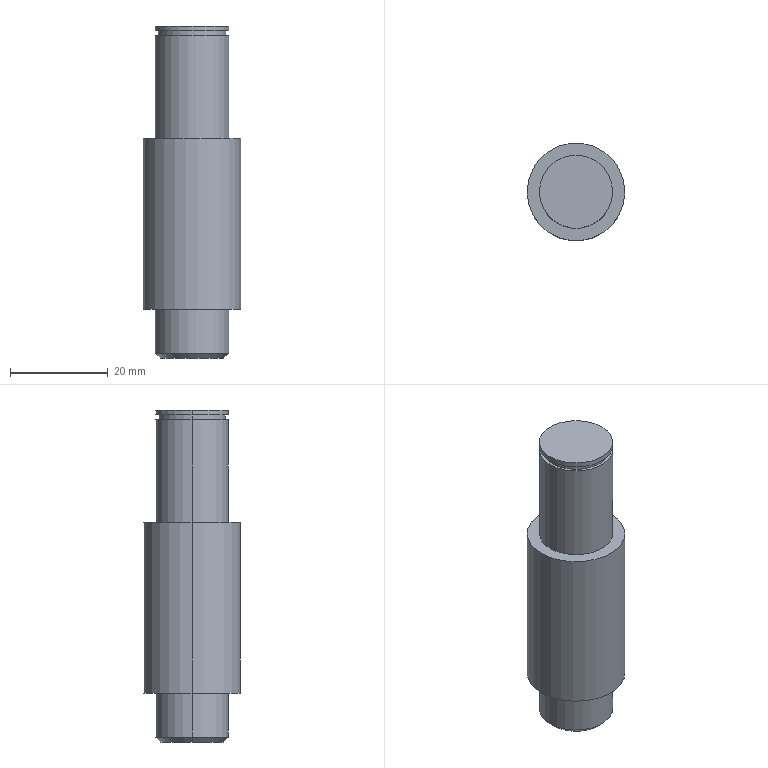Part | STEP file | Tensioning pulley fixing shaft SGN-2-20 | 1 solid | 18 faces | box 20 x 20 x 68 mm | volume 16777 mm3 | cylinder 10 | plane 6 | cone 2 | commonest cylinder face diameters 15 x6 13.8 x2 20 x2
STEP:
#1=CARTESIAN_POINT('',(0.,0.,0.));
#2=DIRECTION('',(0.,0.,1.));
#3=DIRECTION('',(1.,0.,0.));
#4=AXIS2_PLACEMENT_3D('',#1,#2,#3);
#5=CARTESIAN_POINT('',(-6.5,0.,0.));
#6=VERTEX_POINT('',#5);
#7=CARTESIAN_POINT('',(6.5,0.,0.));
#8=VERTEX_POINT('',#7);
#9=CARTESIAN_POINT('',(0.,0.,0.));
#10=DIRECTION('',(0.,0.,-1.));
#11=DIRECTION('',(1.,0.,0.));
#12=AXIS2_PLACEMENT_3D('',#9,#10,#11);
#13=CIRCLE('',#12,6.5);
#14=CARTESIAN_POINT('',(0.,0.,1.));
#15=DIRECTION('',(0.,0.,1.));
#16=DIRECTION('',(1.,0.,0.));
#17=AXIS2_PLACEMENT_3D('',#14,#15,#16);
#18=CONICAL_SURFACE('',#17,7.5,0.7854);
#19=CARTESIAN_POINT('',(6.283,-1.));
#20=DIRECTION('',(-1.,0.));
#21=VECTOR('',#20,1.);
#22=LINE('',#19,#21);
#23=(GEOMETRIC_REPRESENTATION_CONTEXT(2)PARAMETRIC_REPRESENTATION_CONTEXT()REPRESENTATION_CONTEXT('',''));
#24=DEFINITIONAL_REPRESENTATION('',(#22),#23);
#25=PCURVE('',#18,#24);
#26=CARTESIAN_POINT('',(0.,0.,0.));
#27=DIRECTION('',(0.,0.,1.));
#28=DIRECTION('',(1.,0.,0.));
#29=AXIS2_PLACEMENT_3D('',#26,#27,#28);
#30=PLANE('',#29);
#31=CARTESIAN_POINT('',(6.5,0.));
#32=CARTESIAN_POINT('',(6.5,-11.258));
#33=CARTESIAN_POINT('',(-3.25,-5.629));
#34=CARTESIAN_POINT('',(-13.,0.));
#35=CARTESIAN_POINT('',(-3.25,5.629));
#36=CARTESIAN_POINT('',(6.5,11.258));
#37=CARTESIAN_POINT('',(6.5,0.));
#38=(BOUNDED_CURVE()B_SPLINE_CURVE(2,(#31,#32,#33,#34,#35,#36,#37),.UNSPECIFIED.,.T.,.F.)B_SPLINE_CURVE_WITH_KNOTS((1,2,2,2,2,1),(-2.094,0.,2.094,4.189,6.283,8.378),.UNSPECIFIED.)CURVE()GEOMETRIC_REPRESENTATION_ITEM()RATIONAL_B_SPLINE_CURVE((1.,0.5,1.,0.5,1.,0.5,1.))REPRESENTATION_ITEM(''));
#39=(GEOMETRIC_REPRESENTATION_CONTEXT(2)PARAMETRIC_REPRESENTATION_CONTEXT()REPRESENTATION_CONTEXT('',''));
#40=DEFINITIONAL_REPRESENTATION('',(#38),#39);
#41=PCURVE('',#30,#40);
#42=SURFACE_CURVE('',#13,(#25,#41),.PCURVE_S1.);
#43=EDGE_CURVE('',#6,#8,#42,.T.);
#44=ORIENTED_EDGE('',*,*,#43,.F.);
#45=CARTESIAN_POINT('',(-7.5,0.,1.));
#46=VERTEX_POINT('',#45);
#47=CARTESIAN_POINT('',(-7.5,0.,1.));
#48=DIRECTION('',(-0.7071,0.,0.7071));
#49=VECTOR('',#48,1.);
#50=LINE('',#47,#49);
#51=CARTESIAN_POINT('',(3.142,0.));
#52=DIRECTION('',(0.,1.));
#53=VECTOR('',#52,1.);
#54=LINE('',#51,#53);
#55=(GEOMETRIC_REPRESENTATION_CONTEXT(2)PARAMETRIC_REPRESENTATION_CONTEXT()REPRESENTATION_CONTEXT('',''));
#56=DEFINITIONAL_REPRESENTATION('',(#54),#55);
#57=PCURVE('',#18,#56);
#58=CARTESIAN_POINT('',(0.,0.,1.));
#59=DIRECTION('',(0.,0.,1.));
#60=DIRECTION('',(1.,0.,0.));
#61=AXIS2_PLACEMENT_3D('',#58,#59,#60);
#62=CONICAL_SURFACE('',#61,7.5,0.7854);
#63=CARTESIAN_POINT('',(3.142,0.));
#64=DIRECTION('',(0.,1.));
#65=VECTOR('',#64,1.);
#66=LINE('',#63,#65);
#67=(GEOMETRIC_REPRESENTATION_CONTEXT(2)PARAMETRIC_REPRESENTATION_CONTEXT()REPRESENTATION_CONTEXT('',''));
#68=DEFINITIONAL_REPRESENTATION('',(#66),#67);
#69=PCURVE('',#62,#68);
#70=SURFACE_CURVE('',#50,(#57,#69),.PCURVE_S1.);
#71=EDGE_CURVE('',#6,#46,#70,.T.);
#72=ORIENTED_EDGE('',*,*,#71,.T.);
#73=CARTESIAN_POINT('',(7.5,0.,1.));
#74=VERTEX_POINT('',#73);
#75=CARTESIAN_POINT('',(0.,0.,1.));
#76=DIRECTION('',(0.,0.,1.));
#77=DIRECTION('',(1.,0.,0.));
#78=AXIS2_PLACEMENT_3D('',#75,#76,#77);
#79=CIRCLE('',#78,7.5);
#80=CARTESIAN_POINT('',(0.,0.));
#81=DIRECTION('',(1.,0.));
#82=VECTOR('',#81,1.);
#83=LINE('',#80,#82);
#84=(GEOMETRIC_REPRESENTATION_CONTEXT(2)PARAMETRIC_REPRESENTATION_CONTEXT()REPRESENTATION_CONTEXT('',''));
#85=DEFINITIONAL_REPRESENTATION('',(#83),#84);
#86=PCURVE('',#18,#85);
#87=CARTESIAN_POINT('',(0.,0.,10.));
#88=DIRECTION('',(0.,0.,-1.));
#89=DIRECTION('',(-1.,0.,0.));
#90=AXIS2_PLACEMENT_3D('',#87,#88,#89);
#91=CYLINDRICAL_SURFACE('',#90,7.5);
#92=CARTESIAN_POINT('',(3.142,9.));
#93=DIRECTION('',(-1.,0.));
#94=VECTOR('',#93,1.);
#95=LINE('',#92,#94);
#96=(GEOMETRIC_REPRESENTATION_CONTEXT(2)PARAMETRIC_REPRESENTATION_CONTEXT()REPRESENTATION_CONTEXT('',''));
#97=DEFINITIONAL_REPRESENTATION('',(#95),#96);
#98=PCURVE('',#91,#97);
#99=SURFACE_CURVE('',#79,(#86,#98),.PCURVE_S1.);
#100=EDGE_CURVE('',#74,#46,#99,.T.);
#101=ORIENTED_EDGE('',*,*,#100,.F.);
#102=CARTESIAN_POINT('',(7.5,0.,1.));
#103=DIRECTION('',(0.7071,0.,0.7071));
#104=VECTOR('',#103,1.);
#105=LINE('',#102,#104);
#106=CARTESIAN_POINT('',(0.,0.));
#107=DIRECTION('',(0.,1.));
#108=VECTOR('',#107,1.);
#109=LINE('',#106,#108);
#110=(GEOMETRIC_REPRESENTATION_CONTEXT(2)PARAMETRIC_REPRESENTATION_CONTEXT()REPRESENTATION_CONTEXT('',''));
#111=DEFINITIONAL_REPRESENTATION('',(#109),#110);
#112=PCURVE('',#18,#111);
#113=CARTESIAN_POINT('',(6.283,0.));
#114=DIRECTION('',(0.,1.));
#115=VECTOR('',#114,1.);
#116=LINE('',#113,#115);
#117=(GEOMETRIC_REPRESENTATION_CONTEXT(2)PARAMETRIC_REPRESENTATION_CONTEXT()REPRESENTATION_CONTEXT('',''));
#118=DEFINITIONAL_REPRESENTATION('',(#116),#117);
#119=PCURVE('',#62,#118);
#120=SURFACE_CURVE('',#105,(#112,#119),.PCURVE_S1.);
#121=EDGE_CURVE('',#8,#74,#120,.T.);
#122=ORIENTED_EDGE('',*,*,#121,.F.);
#123=EDGE_LOOP('',(#44,#72,#101,#122));
#124=FACE_BOUND('',#123,.T.);
#125=ADVANCED_FACE('',(#124),#18,.T.);
#126=CARTESIAN_POINT('',(7.5,0.,68.));
#127=VERTEX_POINT('',#126);
#128=CARTESIAN_POINT('',(-7.5,0.,68.));
#129=VERTEX_POINT('',#128);
#130=CARTESIAN_POINT('',(0.,0.,68.));
#131=DIRECTION('',(0.,0.,1.));
#132=DIRECTION('',(1.,0.,0.));
#133=AXIS2_PLACEMENT_3D('',#130,#131,#132);
#134=CIRCLE('',#133,7.5);
#135=CARTESIAN_POINT('',(0.,0.,68.));
#136=DIRECTION('',(0.,0.,-1.));
#137=DIRECTION('',(-1.,0.,0.));
#138=AXIS2_PLACEMENT_3D('',#135,#136,#137);
#139=CYLINDRICAL_SURFACE('',#138,7.5);
#140=CARTESIAN_POINT('',(3.142,0.));
#141=DIRECTION('',(-1.,0.));
#142=VECTOR('',#141,1.);
#143=LINE('',#140,#142);
#144=(GEOMETRIC_REPRESENTATION_CONTEXT(2)PARAMETRIC_REPRESENTATION_CONTEXT()REPRESENTATION_CONTEXT('',''));
#145=DEFINITIONAL_REPRESENTATION('',(#143),#144);
#146=PCURVE('',#139,#145);
#147=CARTESIAN_POINT('',(0.,0.,68.));
#148=DIRECTION('',(0.,0.,1.));
#149=DIRECTION('',(1.,0.,0.));
#150=AXIS2_PLACEMENT_3D('',#147,#148,#149);
#151=PLANE('',#150);
#152=CARTESIAN_POINT('',(0.,0.));
#153=DIRECTION('',(1.,0.));
#154=AXIS2_PLACEMENT_2D('',#152,#153);
#155=CIRCLE('',#154,7.5);
#156=(GEOMETRIC_REPRESENTATION_CONTEXT(2)PARAMETRIC_REPRESENTATION_CONTEXT()REPRESENTATION_CONTEXT('',''));
#157=DEFINITIONAL_REPRESENTATION('',(#155),#156);
#158=PCURVE('',#151,#157);
#159=SURFACE_CURVE('',#134,(#146,#158),.PCURVE_S1.);
#160=EDGE_CURVE('',#127,#129,#159,.T.);
#161=ORIENTED_EDGE('',*,*,#160,.F.);
#162=CARTESIAN_POINT('',(7.5,0.,67.));
#163=VERTEX_POINT('',#162);
#164=CARTESIAN_POINT('',(7.5,0.,68.));
#165=DIRECTION('',(0.,0.,-1.));
#166=VECTOR('',#165,1.);
#167=LINE('',#164,#166);
#168=CARTESIAN_POINT('',(3.142,0.));
#169=DIRECTION('',(0.,1.));
#170=VECTOR('',#169,1.);
#171=LINE('',#168,#170);
#172=(GEOMETRIC_REPRESENTATION_CONTEXT(2)PARAMETRIC_REPRESENTATION_CONTEXT()REPRESENTATION_CONTEXT('',''));
#173=DEFINITIONAL_REPRESENTATION('',(#171),#172);
#174=PCURVE('',#139,#173);
#175=CARTESIAN_POINT('',(0.,0.,68.));
#176=DIRECTION('',(0.,0.,-1.));
#177=DIRECTION('',(-1.,0.,0.));
#178=AXIS2_PLACEMENT_3D('',#175,#176,#177);
#179=CYLINDRICAL_SURFACE('',#178,7.5);
#180=CARTESIAN_POINT('',(3.142,0.));
#181=DIRECTION('',(0.,1.));
#182=VECTOR('',#181,1.);
#183=LINE('',#180,#182);
#184=(GEOMETRIC_REPRESENTATION_CONTEXT(2)PARAMETRIC_REPRESENTATION_CONTEXT()REPRESENTATION_CONTEXT('',''));
#185=DEFINITIONAL_REPRESENTATION('',(#183),#184);
#186=PCURVE('',#179,#185);
#187=SURFACE_CURVE('',#167,(#174,#186),.PCURVE_S1.);
#188=EDGE_CURVE('',#127,#163,#187,.T.);
#189=ORIENTED_EDGE('',*,*,#188,.T.);
#190=CARTESIAN_POINT('',(-7.5,0.,67.));
#191=VERTEX_POINT('',#190);
#192=CARTESIAN_POINT('',(0.,0.,67.));
#193=DIRECTION('',(0.,0.,1.));
#194=DIRECTION('',(1.,0.,0.));
#195=AXIS2_PLACEMENT_3D('',#192,#193,#194);
#196=CIRCLE('',#195,7.5);
#197=CARTESIAN_POINT('',(3.142,1.));
#198=DIRECTION('',(-1.,0.));
#199=VECTOR('',#198,1.);
#200=LINE('',#197,#199);
#201=(GEOMETRIC_REPRESENTATION_CONTEXT(2)PARAMETRIC_REPRESENTATION_CONTEXT()REPRESENTATION_CONTEXT('',''));
#202=DEFINITIONAL_REPRESENTATION('',(#200),#201);
#203=PCURVE('',#139,#202);
#204=CARTESIAN_POINT('',(0.,0.,67.));
#205=DIRECTION('',(0.,0.,1.));
#206=DIRECTION('',(1.,0.,0.));
#207=AXIS2_PLACEMENT_3D('',#204,#205,#206);
#208=PLANE('',#207);
#209=CARTESIAN_POINT('',(0.,0.));
#210=DIRECTION('',(1.,0.));
#211=AXIS2_PLACEMENT_2D('',#209,#210);
#212=CIRCLE('',#211,7.5);
#213=(GEOMETRIC_REPRESENTATION_CONTEXT(2)PARAMETRIC_REPRESENTATION_CONTEXT()REPRESENTATION_CONTEXT('',''));
#214=DEFINITIONAL_REPRESENTATION('',(#212),#213);
#215=PCURVE('',#208,#214);
#216=SURFACE_CURVE('',#196,(#203,#215),.PCURVE_S1.);
#217=EDGE_CURVE('',#163,#191,#216,.T.);
#218=ORIENTED_EDGE('',*,*,#217,.T.);
#219=CARTESIAN_POINT('',(-7.5,0.,68.));
#220=DIRECTION('',(0.,0.,-1.));
#221=VECTOR('',#220,1.);
#222=LINE('',#219,#221);
#223=CARTESIAN_POINT('',(0.,0.));
#224=DIRECTION('',(0.,1.));
#225=VECTOR('',#224,1.);
#226=LINE('',#223,#225);
#227=(GEOMETRIC_REPRESENTATION_CONTEXT(2)PARAMETRIC_REPRESENTATION_CONTEXT()REPRESENTATION_CONTEXT('',''));
#228=DEFINITIONAL_REPRESENTATION('',(#226),#227);
#229=PCURVE('',#139,#228);
#230=CARTESIAN_POINT('',(6.283,0.));
#231=DIRECTION('',(0.,1.));
#232=VECTOR('',#231,1.);
#233=LINE('',#230,#232);
#234=(GEOMETRIC_REPRESENTATION_CONTEXT(2)PARAMETRIC_REPRESENTATION_CONTEXT()REPRESENTATION_CONTEXT('',''));
#235=DEFINITIONAL_REPRESENTATION('',(#233),#234);
#236=PCURVE('',#179,#235);
#237=SURFACE_CURVE('',#222,(#229,#236),.PCURVE_S1.);
#238=EDGE_CURVE('',#129,#191,#237,.T.);
#239=ORIENTED_EDGE('',*,*,#238,.F.);
#240=EDGE_LOOP('',(#161,#189,#218,#239));
#241=FACE_BOUND('',#240,.T.);
#242=ADVANCED_FACE('',(#241),#139,.T.);
#243=CARTESIAN_POINT('',(6.9,0.,66.));
#244=VERTEX_POINT('',#243);
#245=CARTESIAN_POINT('',(-6.9,0.,66.));
#246=VERTEX_POINT('',#245);
#247=CARTESIAN_POINT('',(0.,0.,66.));
#248=DIRECTION('',(0.,0.,1.));
#249=DIRECTION('',(1.,0.,0.));
#250=AXIS2_PLACEMENT_3D('',#247,#248,#249);
#251=CIRCLE('',#250,6.9);
#252=CARTESIAN_POINT('',(0.,0.,66.));
#253=DIRECTION('',(0.,0.,1.));
#254=DIRECTION('',(1.,0.,0.));
#255=AXIS2_PLACEMENT_3D('',#252,#253,#254);
#256=CYLINDRICAL_SURFACE('',#255,6.9);
#257=CARTESIAN_POINT('',(0.,0.));
#258=DIRECTION('',(1.,0.));
#259=VECTOR('',#258,1.);
#260=LINE('',#257,#259);
#261=(GEOMETRIC_REPRESENTATION_CONTEXT(2)PARAMETRIC_REPRESENTATION_CONTEXT()REPRESENTATION_CONTEXT('',''));
#262=DEFINITIONAL_REPRESENTATION('',(#260),#261);
#263=PCURVE('',#256,#262);
#264=CARTESIAN_POINT('',(0.,0.,66.));
#265=DIRECTION('',(0.,0.,1.));
#266=DIRECTION('',(1.,0.,0.));
#267=AXIS2_PLACEMENT_3D('',#264,#265,#266);
#268=PLANE('',#267);
#269=CARTESIAN_POINT('',(0.,0.));
#270=DIRECTION('',(1.,0.));
#271=AXIS2_PLACEMENT_2D('',#269,#270);
#272=CIRCLE('',#271,6.9);
#273=(GEOMETRIC_REPRESENTATION_CONTEXT(2)PARAMETRIC_REPRESENTATION_CONTEXT()REPRESENTATION_CONTEXT('',''));
#274=DEFINITIONAL_REPRESENTATION('',(#272),#273);
#275=PCURVE('',#268,#274);
#276=SURFACE_CURVE('',#251,(#263,#275),.PCURVE_S1.);
#277=EDGE_CURVE('',#244,#246,#276,.T.);
#278=ORIENTED_EDGE('',*,*,#277,.T.);
#279=CARTESIAN_POINT('',(-6.9,0.,67.));
#280=VERTEX_POINT('',#279);
#281=CARTESIAN_POINT('',(-6.9,0.,66.));
#282=DIRECTION('',(0.,0.,1.));
#283=VECTOR('',#282,1.);
#284=LINE('',#281,#283);
#285=CARTESIAN_POINT('',(3.142,0.));
#286=DIRECTION('',(0.,1.));
#287=VECTOR('',#286,1.);
#288=LINE('',#285,#287);
#289=(GEOMETRIC_REPRESENTATION_CONTEXT(2)PARAMETRIC_REPRESENTATION_CONTEXT()REPRESENTATION_CONTEXT('',''));
#290=DEFINITIONAL_REPRESENTATION('',(#288),#289);
#291=PCURVE('',#256,#290);
#292=CARTESIAN_POINT('',(0.,0.,66.));
#293=DIRECTION('',(0.,0.,1.));
#294=DIRECTION('',(1.,0.,0.));
#295=AXIS2_PLACEMENT_3D('',#292,#293,#294);
#296=CYLINDRICAL_SURFACE('',#295,6.9);
#297=CARTESIAN_POINT('',(3.142,0.));
#298=DIRECTION('',(0.,1.));
#299=VECTOR('',#298,1.);
#300=LINE('',#297,#299);
#301=(GEOMETRIC_REPRESENTATION_CONTEXT(2)PARAMETRIC_REPRESENTATION_CONTEXT()REPRESENTATION_CONTEXT('',''));
#302=DEFINITIONAL_REPRESENTATION('',(#300),#301);
#303=PCURVE('',#296,#302);
#304=SURFACE_CURVE('',#284,(#291,#303),.PCURVE_S1.);
#305=EDGE_CURVE('',#246,#280,#304,.T.);
#306=ORIENTED_EDGE('',*,*,#305,.T.);
#307=CARTESIAN_POINT('',(6.9,0.,67.));
#308=VERTEX_POINT('',#307);
#309=CARTESIAN_POINT('',(0.,0.,67.));
#310=DIRECTION('',(0.,0.,1.));
#311=DIRECTION('',(1.,0.,0.));
#312=AXIS2_PLACEMENT_3D('',#309,#310,#311);
#313=CIRCLE('',#312,6.9);
#314=CARTESIAN_POINT('',(0.,1.));
#315=DIRECTION('',(1.,0.));
#316=VECTOR('',#315,1.);
#317=LINE('',#314,#316);
#318=(GEOMETRIC_REPRESENTATION_CONTEXT(2)PARAMETRIC_REPRESENTATION_CONTEXT()REPRESENTATION_CONTEXT('',''));
#319=DEFINITIONAL_REPRESENTATION('',(#317),#318);
#320=PCURVE('',#256,#319);
#321=CARTESIAN_POINT('',(0.,0.));
#322=DIRECTION('',(1.,0.));
#323=AXIS2_PLACEMENT_2D('',#321,#322);
#324=CIRCLE('',#323,6.9);
#325=(GEOMETRIC_REPRESENTATION_CONTEXT(2)PARAMETRIC_REPRESENTATION_CONTEXT()REPRESENTATION_CONTEXT('',''));
#326=DEFINITIONAL_REPRESENTATION('',(#324),#325);
#327=PCURVE('',#208,#326);
#328=SURFACE_CURVE('',#313,(#320,#327),.PCURVE_S1.);
#329=EDGE_CURVE('',#308,#280,#328,.T.);
#330=ORIENTED_EDGE('',*,*,#329,.F.);
#331=CARTESIAN_POINT('',(6.9,0.,66.));
#332=DIRECTION('',(0.,0.,1.));
#333=VECTOR('',#332,1.);
#334=LINE('',#331,#333);
#335=CARTESIAN_POINT('',(0.,0.));
#336=DIRECTION('',(0.,1.));
#337=VECTOR('',#336,1.);
#338=LINE('',#335,#337);
#339=(GEOMETRIC_REPRESENTATION_CONTEXT(2)PARAMETRIC_REPRESENTATION_CONTEXT()REPRESENTATION_CONTEXT('',''));
#340=DEFINITIONAL_REPRESENTATION('',(#338),#339);
#341=PCURVE('',#256,#340);
#342=CARTESIAN_POINT('',(6.283,0.));
#343=DIRECTION('',(0.,1.));
#344=VECTOR('',#343,1.);
#345=LINE('',#342,#344);
#346=(GEOMETRIC_REPRESENTATION_CONTEXT(2)PARAMETRIC_REPRESENTATION_CONTEXT()REPRESENTATION_CONTEXT('',''));
#347=DEFINITIONAL_REPRESENTATION('',(#345),#346);
#348=PCURVE('',#296,#347);
#349=SURFACE_CURVE('',#334,(#341,#348),.PCURVE_S1.);
#350=EDGE_CURVE('',#244,#308,#349,.T.);
#351=ORIENTED_EDGE('',*,*,#350,.F.);
#352=EDGE_LOOP('',(#278,#306,#330,#351));
#353=FACE_BOUND('',#352,.T.);
#354=ADVANCED_FACE('',(#353),#256,.T.);
#355=CARTESIAN_POINT('',(10.,0.,45.));
#356=VERTEX_POINT('',#355);
#357=CARTESIAN_POINT('',(-10.,0.,45.));
#358=VERTEX_POINT('',#357);
#359=CARTESIAN_POINT('',(0.,0.,45.));
#360=DIRECTION('',(0.,0.,1.));
#361=DIRECTION('',(1.,0.,0.));
#362=AXIS2_PLACEMENT_3D('',#359,#360,#361);
#363=CIRCLE('',#362,10.);
#364=CARTESIAN_POINT('',(0.,0.,45.));
#365=DIRECTION('',(0.,0.,-1.));
#366=DIRECTION('',(-1.,0.,0.));
#367=AXIS2_PLACEMENT_3D('',#364,#365,#366);
#368=CYLINDRICAL_SURFACE('',#367,10.);
#369=CARTESIAN_POINT('',(3.142,0.));
#370=DIRECTION('',(-1.,0.));
#371=VECTOR('',#370,1.);
#372=LINE('',#369,#371);
#373=(GEOMETRIC_REPRESENTATION_CONTEXT(2)PARAMETRIC_REPRESENTATION_CONTEXT()REPRESENTATION_CONTEXT('',''));
#374=DEFINITIONAL_REPRESENTATION('',(#372),#373);
#375=PCURVE('',#368,#374);
#376=CARTESIAN_POINT('',(0.,0.,45.));
#377=DIRECTION('',(0.,0.,1.));
#378=DIRECTION('',(1.,0.,0.));
#379=AXIS2_PLACEMENT_3D('',#376,#377,#378);
#380=PLANE('',#379);
#381=CARTESIAN_POINT('',(0.,0.));
#382=DIRECTION('',(1.,0.));
#383=AXIS2_PLACEMENT_2D('',#381,#382);
#384=CIRCLE('',#383,10.);
#385=(GEOMETRIC_REPRESENTATION_CONTEXT(2)PARAMETRIC_REPRESENTATION_CONTEXT()REPRESENTATION_CONTEXT('',''));
#386=DEFINITIONAL_REPRESENTATION('',(#384),#385);
#387=PCURVE('',#380,#386);
#388=SURFACE_CURVE('',#363,(#375,#387),.PCURVE_S1.);
#389=EDGE_CURVE('',#356,#358,#388,.T.);
#390=ORIENTED_EDGE('',*,*,#389,.F.);
#391=CARTESIAN_POINT('',(10.,0.,10.));
#392=VERTEX_POINT('',#391);
#393=CARTESIAN_POINT('',(10.,0.,45.));
#394=DIRECTION('',(0.,0.,-1.));
#395=VECTOR('',#394,1.);
#396=LINE('',#393,#395);
#397=CARTESIAN_POINT('',(3.142,0.));
#398=DIRECTION('',(0.,1.));
#399=VECTOR('',#398,1.);
#400=LINE('',#397,#399);
#401=(GEOMETRIC_REPRESENTATION_CONTEXT(2)PARAMETRIC_REPRESENTATION_CONTEXT()REPRESENTATION_CONTEXT('',''));
#402=DEFINITIONAL_REPRESENTATION('',(#400),#401);
#403=PCURVE('',#368,#402);
#404=CARTESIAN_POINT('',(0.,0.,45.));
#405=DIRECTION('',(0.,0.,-1.));
#406=DIRECTION('',(-1.,0.,0.));
#407=AXIS2_PLACEMENT_3D('',#404,#405,#406);
#408=CYLINDRICAL_SURFACE('',#407,10.);
#409=CARTESIAN_POINT('',(3.142,0.));
#410=DIRECTION('',(0.,1.));
#411=VECTOR('',#410,1.);
#412=LINE('',#409,#411);
#413=(GEOMETRIC_REPRESENTATION_CONTEXT(2)PARAMETRIC_REPRESENTATION_CONTEXT()REPRESENTATION_CONTEXT('',''));
#414=DEFINITIONAL_REPRESENTATION('',(#412),#413);
#415=PCURVE('',#408,#414);
#416=SURFACE_CURVE('',#396,(#403,#415),.PCURVE_S1.);
#417=EDGE_CURVE('',#356,#392,#416,.T.);
#418=ORIENTED_EDGE('',*,*,#417,.T.);
#419=CARTESIAN_POINT('',(-10.,0.,10.));
#420=VERTEX_POINT('',#419);
#421=CARTESIAN_POINT('',(0.,0.,10.));
#422=DIRECTION('',(0.,0.,1.));
#423=DIRECTION('',(1.,0.,0.));
#424=AXIS2_PLACEMENT_3D('',#421,#422,#423);
#425=CIRCLE('',#424,10.);
#426=CARTESIAN_POINT('',(3.142,35.));
#427=DIRECTION('',(-1.,0.));
#428=VECTOR('',#427,1.);
#429=LINE('',#426,#428);
#430=(GEOMETRIC_REPRESENTATION_CONTEXT(2)PARAMETRIC_REPRESENTATION_CONTEXT()REPRESENTATION_CONTEXT('',''));
#431=DEFINITIONAL_REPRESENTATION('',(#429),#430);
#432=PCURVE('',#368,#431);
#433=CARTESIAN_POINT('',(0.,0.,10.));
#434=DIRECTION('',(0.,0.,1.));
#435=DIRECTION('',(1.,0.,0.));
#436=AXIS2_PLACEMENT_3D('',#433,#434,#435);
#437=PLANE('',#436);
#438=CARTESIAN_POINT('',(0.,0.));
#439=DIRECTION('',(1.,0.));
#440=AXIS2_PLACEMENT_2D('',#438,#439);
#441=CIRCLE('',#440,10.);
#442=(GEOMETRIC_REPRESENTATION_CONTEXT(2)PARAMETRIC_REPRESENTATION_CONTEXT()REPRESENTATION_CONTEXT('',''));
#443=DEFINITIONAL_REPRESENTATION('',(#441),#442);
#444=PCURVE('',#437,#443);
#445=SURFACE_CURVE('',#425,(#432,#444),.PCURVE_S1.);
#446=EDGE_CURVE('',#392,#420,#445,.T.);
#447=ORIENTED_EDGE('',*,*,#446,.T.);
#448=CARTESIAN_POINT('',(-10.,0.,45.));
#449=DIRECTION('',(0.,0.,-1.));
#450=VECTOR('',#449,1.);
#451=LINE('',#448,#450);
#452=CARTESIAN_POINT('',(0.,0.));
#453=DIRECTION('',(0.,1.));
#454=VECTOR('',#453,1.);
#455=LINE('',#452,#454);
#456=(GEOMETRIC_REPRESENTATION_CONTEXT(2)PARAMETRIC_REPRESENTATION_CONTEXT()REPRESENTATION_CONTEXT('',''));
#457=DEFINITIONAL_REPRESENTATION('',(#455),#456);
#458=PCURVE('',#368,#457);
#459=CARTESIAN_POINT('',(6.283,0.));
#460=DIRECTION('',(0.,1.));
#461=VECTOR('',#460,1.);
#462=LINE('',#459,#461);
#463=(GEOMETRIC_REPRESENTATION_CONTEXT(2)PARAMETRIC_REPRESENTATION_CONTEXT()REPRESENTATION_CONTEXT('',''));
#464=DEFINITIONAL_REPRESENTATION('',(#462),#463);
#465=PCURVE('',#408,#464);
#466=SURFACE_CURVE('',#451,(#458,#465),.PCURVE_S1.);
#467=EDGE_CURVE('',#358,#420,#466,.T.);
#468=ORIENTED_EDGE('',*,*,#467,.F.);
#469=EDGE_LOOP('',(#390,#418,#447,#468));
#470=FACE_BOUND('',#469,.T.);
#471=ADVANCED_FACE('',(#470),#368,.T.);
#472=CARTESIAN_POINT('',(7.5,0.,10.));
#473=VERTEX_POINT('',#472);
#474=CARTESIAN_POINT('',(-7.5,0.,10.));
#475=VERTEX_POINT('',#474);
#476=CARTESIAN_POINT('',(0.,0.,10.));
#477=DIRECTION('',(0.,0.,1.));
#478=DIRECTION('',(1.,0.,0.));
#479=AXIS2_PLACEMENT_3D('',#476,#477,#478);
#480=CIRCLE('',#479,7.5);
#481=CARTESIAN_POINT('',(3.142,0.));
#482=DIRECTION('',(-1.,0.));
#483=VECTOR('',#482,1.);
#484=LINE('',#481,#483);
#485=(GEOMETRIC_REPRESENTATION_CONTEXT(2)PARAMETRIC_REPRESENTATION_CONTEXT()REPRESENTATION_CONTEXT('',''));
#486=DEFINITIONAL_REPRESENTATION('',(#484),#485);
#487=PCURVE('',#91,#486);
#488=CARTESIAN_POINT('',(0.,0.));
#489=DIRECTION('',(1.,0.));
#490=AXIS2_PLACEMENT_2D('',#488,#489);
#491=CIRCLE('',#490,7.5);
#492=(GEOMETRIC_REPRESENTATION_CONTEXT(2)PARAMETRIC_REPRESENTATION_CONTEXT()REPRESENTATION_CONTEXT('',''));
#493=DEFINITIONAL_REPRESENTATION('',(#491),#492);
#494=PCURVE('',#437,#493);
#495=SURFACE_CURVE('',#480,(#487,#494),.PCURVE_S1.);
#496=EDGE_CURVE('',#473,#475,#495,.T.);
#497=ORIENTED_EDGE('',*,*,#496,.F.);
#498=CARTESIAN_POINT('',(7.5,0.,10.));
#499=DIRECTION('',(0.,0.,-1.));
#500=VECTOR('',#499,1.);
#501=LINE('',#498,#500);
#502=CARTESIAN_POINT('',(3.142,0.));
#503=DIRECTION('',(0.,1.));
#504=VECTOR('',#503,1.);
#505=LINE('',#502,#504);
#506=(GEOMETRIC_REPRESENTATION_CONTEXT(2)PARAMETRIC_REPRESENTATION_CONTEXT()REPRESENTATION_CONTEXT('',''));
#507=DEFINITIONAL_REPRESENTATION('',(#505),#506);
#508=PCURVE('',#91,#507);
#509=CARTESIAN_POINT('',(0.,0.,10.));
#510=DIRECTION('',(0.,0.,-1.));
#511=DIRECTION('',(-1.,0.,0.));
#512=AXIS2_PLACEMENT_3D('',#509,#510,#511);
#513=CYLINDRICAL_SURFACE('',#512,7.5);
#514=CARTESIAN_POINT('',(3.142,0.));
#515=DIRECTION('',(0.,1.));
#516=VECTOR('',#515,1.);
#517=LINE('',#514,#516);
#518=(GEOMETRIC_REPRESENTATION_CONTEXT(2)PARAMETRIC_REPRESENTATION_CONTEXT()REPRESENTATION_CONTEXT('',''));
#519=DEFINITIONAL_REPRESENTATION('',(#517),#518);
#520=PCURVE('',#513,#519);
#521=SURFACE_CURVE('',#501,(#508,#520),.PCURVE_S1.);
#522=EDGE_CURVE('',#473,#74,#521,.T.);
#523=ORIENTED_EDGE('',*,*,#522,.T.);
#524=ORIENTED_EDGE('',*,*,#100,.T.);
#525=CARTESIAN_POINT('',(-7.5,0.,10.));
#526=DIRECTION('',(0.,0.,-1.));
#527=VECTOR('',#526,1.);
#528=LINE('',#525,#527);
#529=CARTESIAN_POINT('',(0.,0.));
#530=DIRECTION('',(0.,1.));
#531=VECTOR('',#530,1.);
#532=LINE('',#529,#531);
#533=(GEOMETRIC_REPRESENTATION_CONTEXT(2)PARAMETRIC_REPRESENTATION_CONTEXT()REPRESENTATION_CONTEXT('',''));
#534=DEFINITIONAL_REPRESENTATION('',(#532),#533);
#535=PCURVE('',#91,#534);
#536=CARTESIAN_POINT('',(6.283,0.));
#537=DIRECTION('',(0.,1.));
#538=VECTOR('',#537,1.);
#539=LINE('',#536,#538);
#540=(GEOMETRIC_REPRESENTATION_CONTEXT(2)PARAMETRIC_REPRESENTATION_CONTEXT()REPRESENTATION_CONTEXT('',''));
#541=DEFINITIONAL_REPRESENTATION('',(#539),#540);
#542=PCURVE('',#513,#541);
#543=SURFACE_CURVE('',#528,(#535,#542),.PCURVE_S1.);
#544=EDGE_CURVE('',#475,#46,#543,.T.);
#545=ORIENTED_EDGE('',*,*,#544,.F.);
#546=EDGE_LOOP('',(#497,#523,#524,#545));
#547=FACE_BOUND('',#546,.T.);
#548=ADVANCED_FACE('',(#547),#91,.T.);
#549=CARTESIAN_POINT('',(7.5,0.,66.));
#550=VERTEX_POINT('',#549);
#551=CARTESIAN_POINT('',(-7.5,0.,66.));
#552=VERTEX_POINT('',#551);
#553=CARTESIAN_POINT('',(0.,0.,66.));
#554=DIRECTION('',(0.,0.,1.));
#555=DIRECTION('',(1.,0.,0.));
#556=AXIS2_PLACEMENT_3D('',#553,#554,#555);
#557=CIRCLE('',#556,7.5);
#558=CARTESIAN_POINT('',(0.,0.,68.));
#559=DIRECTION('',(0.,0.,-1.));
#560=DIRECTION('',(-1.,0.,0.));
#561=AXIS2_PLACEMENT_3D('',#558,#559,#560);
#562=CYLINDRICAL_SURFACE('',#561,7.5);
#563=CARTESIAN_POINT('',(3.142,2.));
#564=DIRECTION('',(-1.,0.));
#565=VECTOR('',#564,1.);
#566=LINE('',#563,#565);
#567=(GEOMETRIC_REPRESENTATION_CONTEXT(2)PARAMETRIC_REPRESENTATION_CONTEXT()REPRESENTATION_CONTEXT('',''));
#568=DEFINITIONAL_REPRESENTATION('',(#566),#567);
#569=PCURVE('',#562,#568);
#570=CARTESIAN_POINT('',(0.,0.));
#571=DIRECTION('',(1.,0.));
#572=AXIS2_PLACEMENT_2D('',#570,#571);
#573=CIRCLE('',#572,7.5);
#574=(GEOMETRIC_REPRESENTATION_CONTEXT(2)PARAMETRIC_REPRESENTATION_CONTEXT()REPRESENTATION_CONTEXT('',''));
#575=DEFINITIONAL_REPRESENTATION('',(#573),#574);
#576=PCURVE('',#268,#575);
#577=SURFACE_CURVE('',#557,(#569,#576),.PCURVE_S1.);
#578=EDGE_CURVE('',#550,#552,#577,.T.);
#579=ORIENTED_EDGE('',*,*,#578,.F.);
#580=CARTESIAN_POINT('',(7.5,0.,45.));
#581=VERTEX_POINT('',#580);
#582=CARTESIAN_POINT('',(7.5,0.,68.));
#583=DIRECTION('',(0.,0.,-1.));
#584=VECTOR('',#583,1.);
#585=LINE('',#582,#584);
#586=CARTESIAN_POINT('',(3.142,0.));
#587=DIRECTION('',(0.,1.));
#588=VECTOR('',#587,1.);
#589=LINE('',#586,#588);
#590=(GEOMETRIC_REPRESENTATION_CONTEXT(2)PARAMETRIC_REPRESENTATION_CONTEXT()REPRESENTATION_CONTEXT('',''));
#591=DEFINITIONAL_REPRESENTATION('',(#589),#590);
#592=PCURVE('',#562,#591);
#593=CARTESIAN_POINT('',(0.,0.,68.));
#594=DIRECTION('',(0.,0.,-1.));
#595=DIRECTION('',(-1.,0.,0.));
#596=AXIS2_PLACEMENT_3D('',#593,#594,#595);
#597=CYLINDRICAL_SURFACE('',#596,7.5);
#598=CARTESIAN_POINT('',(3.142,0.));
#599=DIRECTION('',(0.,1.));
#600=VECTOR('',#599,1.);
#601=LINE('',#598,#600);
#602=(GEOMETRIC_REPRESENTATION_CONTEXT(2)PARAMETRIC_REPRESENTATION_CONTEXT()REPRESENTATION_CONTEXT('',''));
#603=DEFINITIONAL_REPRESENTATION('',(#601),#602);
#604=PCURVE('',#597,#603);
#605=SURFACE_CURVE('',#585,(#592,#604),.PCURVE_S1.);
#606=EDGE_CURVE('',#550,#581,#605,.T.);
#607=ORIENTED_EDGE('',*,*,#606,.T.);
#608=CARTESIAN_POINT('',(-7.5,0.,45.));
#609=VERTEX_POINT('',#608);
#610=CARTESIAN_POINT('',(0.,0.,45.));
#611=DIRECTION('',(0.,0.,1.));
#612=DIRECTION('',(1.,0.,0.));
#613=AXIS2_PLACEMENT_3D('',#610,#611,#612);
#614=CIRCLE('',#613,7.5);
#615=CARTESIAN_POINT('',(3.142,23.));
#616=DIRECTION('',(-1.,0.));
#617=VECTOR('',#616,1.);
#618=LINE('',#615,#617);
#619=(GEOMETRIC_REPRESENTATION_CONTEXT(2)PARAMETRIC_REPRESENTATION_CONTEXT()REPRESENTATION_CONTEXT('',''));
#620=DEFINITIONAL_REPRESENTATION('',(#618),#619);
#621=PCURVE('',#562,#620);
#622=CARTESIAN_POINT('',(0.,0.));
#623=DIRECTION('',(1.,0.));
#624=AXIS2_PLACEMENT_2D('',#622,#623);
#625=CIRCLE('',#624,7.5);
#626=(GEOMETRIC_REPRESENTATION_CONTEXT(2)PARAMETRIC_REPRESENTATION_CONTEXT()REPRESENTATION_CONTEXT('',''));
#627=DEFINITIONAL_REPRESENTATION('',(#625),#626);
#628=PCURVE('',#380,#627);
#629=SURFACE_CURVE('',#614,(#621,#628),.PCURVE_S1.);
#630=EDGE_CURVE('',#581,#609,#629,.T.);
#631=ORIENTED_EDGE('',*,*,#630,.T.);
#632=CARTESIAN_POINT('',(-7.5,0.,68.));
#633=DIRECTION('',(0.,0.,-1.));
#634=VECTOR('',#633,1.);
#635=LINE('',#632,#634);
#636=CARTESIAN_POINT('',(0.,0.));
#637=DIRECTION('',(0.,1.));
#638=VECTOR('',#637,1.);
#639=LINE('',#636,#638);
#640=(GEOMETRIC_REPRESENTATION_CONTEXT(2)PARAMETRIC_REPRESENTATION_CONTEXT()REPRESENTATION_CONTEXT('',''));
#641=DEFINITIONAL_REPRESENTATION('',(#639),#640);
#642=PCURVE('',#562,#641);
#643=CARTESIAN_POINT('',(6.283,0.));
#644=DIRECTION('',(0.,1.));
#645=VECTOR('',#644,1.);
#646=LINE('',#643,#645);
#647=(GEOMETRIC_REPRESENTATION_CONTEXT(2)PARAMETRIC_REPRESENTATION_CONTEXT()REPRESENTATION_CONTEXT('',''));
#648=DEFINITIONAL_REPRESENTATION('',(#646),#647);
#649=PCURVE('',#597,#648);
#650=SURFACE_CURVE('',#635,(#642,#649),.PCURVE_S1.);
#651=EDGE_CURVE('',#552,#609,#650,.T.);
#652=ORIENTED_EDGE('',*,*,#651,.F.);
#653=EDGE_LOOP('',(#579,#607,#631,#652));
#654=FACE_BOUND('',#653,.T.);
#655=ADVANCED_FACE('',(#654),#562,.T.);
#656=ORIENTED_EDGE('',*,*,#606,.F.);
#657=CARTESIAN_POINT('',(0.,0.,66.));
#658=DIRECTION('',(0.,0.,1.));
#659=DIRECTION('',(1.,0.,0.));
#660=AXIS2_PLACEMENT_3D('',#657,#658,#659);
#661=CIRCLE('',#660,7.5);
#662=CARTESIAN_POINT('',(9.425,2.));
#663=DIRECTION('',(-1.,0.));
#664=VECTOR('',#663,1.);
#665=LINE('',#662,#664);
#666=(GEOMETRIC_REPRESENTATION_CONTEXT(2)PARAMETRIC_REPRESENTATION_CONTEXT()REPRESENTATION_CONTEXT('',''));
#667=DEFINITIONAL_REPRESENTATION('',(#665),#666);
#668=PCURVE('',#597,#667);
#669=CARTESIAN_POINT('',(0.,0.));
#670=DIRECTION('',(1.,0.));
#671=AXIS2_PLACEMENT_2D('',#669,#670);
#672=CIRCLE('',#671,7.5);
#673=(GEOMETRIC_REPRESENTATION_CONTEXT(2)PARAMETRIC_REPRESENTATION_CONTEXT()REPRESENTATION_CONTEXT('',''));
#674=DEFINITIONAL_REPRESENTATION('',(#672),#673);
#675=PCURVE('',#268,#674);
#676=SURFACE_CURVE('',#661,(#668,#675),.PCURVE_S1.);
#677=EDGE_CURVE('',#552,#550,#676,.T.);
#678=ORIENTED_EDGE('',*,*,#677,.F.);
#679=ORIENTED_EDGE('',*,*,#651,.T.);
#680=CARTESIAN_POINT('',(0.,0.,45.));
#681=DIRECTION('',(0.,0.,1.));
#682=DIRECTION('',(1.,0.,0.));
#683=AXIS2_PLACEMENT_3D('',#680,#681,#682);
#684=CIRCLE('',#683,7.5);
#685=CARTESIAN_POINT('',(9.425,23.));
#686=DIRECTION('',(-1.,0.));
#687=VECTOR('',#686,1.);
#688=LINE('',#685,#687);
#689=(GEOMETRIC_REPRESENTATION_CONTEXT(2)PARAMETRIC_REPRESENTATION_CONTEXT()REPRESENTATION_CONTEXT('',''));
#690=DEFINITIONAL_REPRESENTATION('',(#688),#689);
#691=PCURVE('',#597,#690);
#692=CARTESIAN_POINT('',(0.,0.));
#693=DIRECTION('',(1.,0.));
#694=AXIS2_PLACEMENT_2D('',#692,#693);
#695=CIRCLE('',#694,7.5);
#696=(GEOMETRIC_REPRESENTATION_CONTEXT(2)PARAMETRIC_REPRESENTATION_CONTEXT()REPRESENTATION_CONTEXT('',''));
#697=DEFINITIONAL_REPRESENTATION('',(#695),#696);
#698=PCURVE('',#380,#697);
#699=SURFACE_CURVE('',#684,(#691,#698),.PCURVE_S1.);
#700=EDGE_CURVE('',#609,#581,#699,.T.);
#701=ORIENTED_EDGE('',*,*,#700,.T.);
#702=EDGE_LOOP('',(#656,#678,#679,#701));
#703=FACE_BOUND('',#702,.T.);
#704=ADVANCED_FACE('',(#703),#597,.T.);
#705=ORIENTED_EDGE('',*,*,#522,.F.);
#706=CARTESIAN_POINT('',(0.,0.,10.));
#707=DIRECTION('',(0.,0.,1.));
#708=DIRECTION('',(1.,0.,0.));
#709=AXIS2_PLACEMENT_3D('',#706,#707,#708);
#710=CIRCLE('',#709,7.5);
#711=CARTESIAN_POINT('',(9.425,0.));
#712=DIRECTION('',(-1.,0.));
#713=VECTOR('',#712,1.);
#714=LINE('',#711,#713);
#715=(GEOMETRIC_REPRESENTATION_CONTEXT(2)PARAMETRIC_REPRESENTATION_CONTEXT()REPRESENTATION_CONTEXT('',''));
#716=DEFINITIONAL_REPRESENTATION('',(#714),#715);
#717=PCURVE('',#513,#716);
#718=CARTESIAN_POINT('',(0.,0.));
#719=DIRECTION('',(1.,0.));
#720=AXIS2_PLACEMENT_2D('',#718,#719);
#721=CIRCLE('',#720,7.5);
#722=(GEOMETRIC_REPRESENTATION_CONTEXT(2)PARAMETRIC_REPRESENTATION_CONTEXT()REPRESENTATION_CONTEXT('',''));
#723=DEFINITIONAL_REPRESENTATION('',(#721),#722);
#724=PCURVE('',#437,#723);
#725=SURFACE_CURVE('',#710,(#717,#724),.PCURVE_S1.);
#726=EDGE_CURVE('',#475,#473,#725,.T.);
#727=ORIENTED_EDGE('',*,*,#726,.F.);
#728=ORIENTED_EDGE('',*,*,#544,.T.);
#729=CARTESIAN_POINT('',(0.,0.,1.));
#730=DIRECTION('',(0.,0.,1.));
#731=DIRECTION('',(1.,0.,0.));
#732=AXIS2_PLACEMENT_3D('',#729,#730,#731);
#733=CIRCLE('',#732,7.5);
#734=CARTESIAN_POINT('',(9.425,9.));
#735=DIRECTION('',(-1.,0.));
#736=VECTOR('',#735,1.);
#737=LINE('',#734,#736);
#738=(GEOMETRIC_REPRESENTATION_CONTEXT(2)PARAMETRIC_REPRESENTATION_CONTEXT()REPRESENTATION_CONTEXT('',''));
#739=DEFINITIONAL_REPRESENTATION('',(#737),#738);
#740=PCURVE('',#513,#739);
#741=CARTESIAN_POINT('',(0.,0.));
#742=DIRECTION('',(1.,0.));
#743=VECTOR('',#742,1.);
#744=LINE('',#741,#743);
#745=(GEOMETRIC_REPRESENTATION_CONTEXT(2)PARAMETRIC_REPRESENTATION_CONTEXT()REPRESENTATION_CONTEXT('',''));
#746=DEFINITIONAL_REPRESENTATION('',(#744),#745);
#747=PCURVE('',#62,#746);
#748=SURFACE_CURVE('',#733,(#740,#747),.PCURVE_S1.);
#749=EDGE_CURVE('',#46,#74,#748,.T.);
#750=ORIENTED_EDGE('',*,*,#749,.T.);
#751=EDGE_LOOP('',(#705,#727,#728,#750));
#752=FACE_BOUND('',#751,.T.);
#753=ADVANCED_FACE('',(#752),#513,.T.);
#754=CARTESIAN_POINT('',(0.,0.,0.));
#755=DIRECTION('',(0.,0.,-1.));
#756=DIRECTION('',(1.,0.,0.));
#757=AXIS2_PLACEMENT_3D('',#754,#755,#756);
#758=CIRCLE('',#757,6.5);
#759=CARTESIAN_POINT('',(6.5,0.));
#760=CARTESIAN_POINT('',(6.5,-11.258));
#761=CARTESIAN_POINT('',(-3.25,-5.629));
#762=CARTESIAN_POINT('',(-13.,0.));
#763=CARTESIAN_POINT('',(-3.25,5.629));
#764=CARTESIAN_POINT('',(6.5,11.258));
#765=CARTESIAN_POINT('',(6.5,0.));
#766=(BOUNDED_CURVE()B_SPLINE_CURVE(2,(#759,#760,#761,#762,#763,#764,#765),.UNSPECIFIED.,.T.,.F.)B_SPLINE_CURVE_WITH_KNOTS((1,2,2,2,2,1),(-2.094,0.,2.094,4.189,6.283,8.378),.UNSPECIFIED.)CURVE()GEOMETRIC_REPRESENTATION_ITEM()RATIONAL_B_SPLINE_CURVE((1.,0.5,1.,0.5,1.,0.5,1.))REPRESENTATION_ITEM(''));
#767=(GEOMETRIC_REPRESENTATION_CONTEXT(2)PARAMETRIC_REPRESENTATION_CONTEXT()REPRESENTATION_CONTEXT('',''));
#768=DEFINITIONAL_REPRESENTATION('',(#766),#767);
#769=PCURVE('',#30,#768);
#770=CARTESIAN_POINT('',(6.283,-1.));
#771=DIRECTION('',(-1.,0.));
#772=VECTOR('',#771,1.);
#773=LINE('',#770,#772);
#774=(GEOMETRIC_REPRESENTATION_CONTEXT(2)PARAMETRIC_REPRESENTATION_CONTEXT()REPRESENTATION_CONTEXT('',''));
#775=DEFINITIONAL_REPRESENTATION('',(#773),#774);
#776=PCURVE('',#62,#775);
#777=SURFACE_CURVE('',#758,(#769,#776),.PCURVE_S1.);
#778=EDGE_CURVE('',#8,#6,#777,.T.);
#779=ORIENTED_EDGE('',*,*,#778,.T.);
#780=ORIENTED_EDGE('',*,*,#43,.T.);
#781=EDGE_LOOP('',(#779,#780));
#782=FACE_BOUND('',#781,.T.);
#783=ADVANCED_FACE('',(#782),#30,.F.);
#784=ORIENTED_EDGE('',*,*,#417,.F.);
#785=CARTESIAN_POINT('',(0.,0.,45.));
#786=DIRECTION('',(0.,0.,1.));
#787=DIRECTION('',(1.,0.,0.));
#788=AXIS2_PLACEMENT_3D('',#785,#786,#787);
#789=CIRCLE('',#788,10.);
#790=CARTESIAN_POINT('',(9.425,0.));
#791=DIRECTION('',(-1.,0.));
#792=VECTOR('',#791,1.);
#793=LINE('',#790,#792);
#794=(GEOMETRIC_REPRESENTATION_CONTEXT(2)PARAMETRIC_REPRESENTATION_CONTEXT()REPRESENTATION_CONTEXT('',''));
#795=DEFINITIONAL_REPRESENTATION('',(#793),#794);
#796=PCURVE('',#408,#795);
#797=CARTESIAN_POINT('',(0.,0.));
#798=DIRECTION('',(1.,0.));
#799=AXIS2_PLACEMENT_2D('',#797,#798);
#800=CIRCLE('',#799,10.);
#801=(GEOMETRIC_REPRESENTATION_CONTEXT(2)PARAMETRIC_REPRESENTATION_CONTEXT()REPRESENTATION_CONTEXT('',''));
#802=DEFINITIONAL_REPRESENTATION('',(#800),#801);
#803=PCURVE('',#380,#802);
#804=SURFACE_CURVE('',#789,(#796,#803),.PCURVE_S1.);
#805=EDGE_CURVE('',#358,#356,#804,.T.);
#806=ORIENTED_EDGE('',*,*,#805,.F.);
#807=ORIENTED_EDGE('',*,*,#467,.T.);
#808=CARTESIAN_POINT('',(0.,0.,10.));
#809=DIRECTION('',(0.,0.,1.));
#810=DIRECTION('',(1.,0.,0.));
#811=AXIS2_PLACEMENT_3D('',#808,#809,#810);
#812=CIRCLE('',#811,10.);
#813=CARTESIAN_POINT('',(9.425,35.));
#814=DIRECTION('',(-1.,0.));
#815=VECTOR('',#814,1.);
#816=LINE('',#813,#815);
#817=(GEOMETRIC_REPRESENTATION_CONTEXT(2)PARAMETRIC_REPRESENTATION_CONTEXT()REPRESENTATION_CONTEXT('',''));
#818=DEFINITIONAL_REPRESENTATION('',(#816),#817);
#819=PCURVE('',#408,#818);
#820=CARTESIAN_POINT('',(0.,0.));
#821=DIRECTION('',(1.,0.));
#822=AXIS2_PLACEMENT_2D('',#820,#821);
#823=CIRCLE('',#822,10.);
#824=(GEOMETRIC_REPRESENTATION_CONTEXT(2)PARAMETRIC_REPRESENTATION_CONTEXT()REPRESENTATION_CONTEXT('',''));
#825=DEFINITIONAL_REPRESENTATION('',(#823),#824);
#826=PCURVE('',#437,#825);
#827=SURFACE_CURVE('',#812,(#819,#826),.PCURVE_S1.);
#828=EDGE_CURVE('',#420,#392,#827,.T.);
#829=ORIENTED_EDGE('',*,*,#828,.T.);
#830=EDGE_LOOP('',(#784,#806,#807,#829));
#831=FACE_BOUND('',#830,.T.);
#832=ADVANCED_FACE('',(#831),#408,.T.);
#833=ORIENTED_EDGE('',*,*,#700,.F.);
#834=ORIENTED_EDGE('',*,*,#630,.F.);
#835=EDGE_LOOP('',(#833,#834));
#836=FACE_BOUND('',#835,.T.);
#837=ORIENTED_EDGE('',*,*,#805,.T.);
#838=ORIENTED_EDGE('',*,*,#389,.T.);
#839=EDGE_LOOP('',(#837,#838));
#840=FACE_BOUND('',#839,.T.);
#841=ADVANCED_FACE('',(#836,#840),#380,.T.);
#842=ORIENTED_EDGE('',*,*,#726,.T.);
#843=ORIENTED_EDGE('',*,*,#496,.T.);
#844=EDGE_LOOP('',(#842,#843));
#845=FACE_BOUND('',#844,.T.);
#846=ORIENTED_EDGE('',*,*,#828,.F.);
#847=ORIENTED_EDGE('',*,*,#446,.F.);
#848=EDGE_LOOP('',(#846,#847));
#849=FACE_BOUND('',#848,.T.);
#850=ADVANCED_FACE('',(#845,#849),#437,.F.);
#851=ORIENTED_EDGE('',*,*,#277,.F.);
#852=CARTESIAN_POINT('',(0.,0.,66.));
#853=DIRECTION('',(0.,0.,1.));
#854=DIRECTION('',(1.,0.,0.));
#855=AXIS2_PLACEMENT_3D('',#852,#853,#854);
#856=CIRCLE('',#855,6.9);
#857=CARTESIAN_POINT('',(0.,0.));
#858=DIRECTION('',(1.,0.));
#859=AXIS2_PLACEMENT_2D('',#857,#858);
#860=CIRCLE('',#859,6.9);
#861=(GEOMETRIC_REPRESENTATION_CONTEXT(2)PARAMETRIC_REPRESENTATION_CONTEXT()REPRESENTATION_CONTEXT('',''));
#862=DEFINITIONAL_REPRESENTATION('',(#860),#861);
#863=PCURVE('',#268,#862);
#864=CARTESIAN_POINT('',(0.,0.));
#865=DIRECTION('',(1.,0.));
#866=VECTOR('',#865,1.);
#867=LINE('',#864,#866);
#868=(GEOMETRIC_REPRESENTATION_CONTEXT(2)PARAMETRIC_REPRESENTATION_CONTEXT()REPRESENTATION_CONTEXT('',''));
#869=DEFINITIONAL_REPRESENTATION('',(#867),#868);
#870=PCURVE('',#296,#869);
#871=SURFACE_CURVE('',#856,(#863,#870),.PCURVE_S1.);
#872=EDGE_CURVE('',#246,#244,#871,.T.);
#873=ORIENTED_EDGE('',*,*,#872,.F.);
#874=EDGE_LOOP('',(#851,#873));
#875=FACE_BOUND('',#874,.T.);
#876=ORIENTED_EDGE('',*,*,#677,.T.);
#877=ORIENTED_EDGE('',*,*,#578,.T.);
#878=EDGE_LOOP('',(#876,#877));
#879=FACE_BOUND('',#878,.T.);
#880=ADVANCED_FACE('',(#875,#879),#268,.T.);
#881=ORIENTED_EDGE('',*,*,#329,.T.);
#882=CARTESIAN_POINT('',(0.,0.,67.));
#883=DIRECTION('',(0.,0.,1.));
#884=DIRECTION('',(1.,0.,0.));
#885=AXIS2_PLACEMENT_3D('',#882,#883,#884);
#886=CIRCLE('',#885,6.9);
#887=CARTESIAN_POINT('',(0.,0.));
#888=DIRECTION('',(1.,0.));
#889=AXIS2_PLACEMENT_2D('',#887,#888);
#890=CIRCLE('',#889,6.9);
#891=(GEOMETRIC_REPRESENTATION_CONTEXT(2)PARAMETRIC_REPRESENTATION_CONTEXT()REPRESENTATION_CONTEXT('',''));
#892=DEFINITIONAL_REPRESENTATION('',(#890),#891);
#893=PCURVE('',#208,#892);
#894=CARTESIAN_POINT('',(0.,1.));
#895=DIRECTION('',(1.,0.));
#896=VECTOR('',#895,1.);
#897=LINE('',#894,#896);
#898=(GEOMETRIC_REPRESENTATION_CONTEXT(2)PARAMETRIC_REPRESENTATION_CONTEXT()REPRESENTATION_CONTEXT('',''));
#899=DEFINITIONAL_REPRESENTATION('',(#897),#898);
#900=PCURVE('',#296,#899);
#901=SURFACE_CURVE('',#886,(#893,#900),.PCURVE_S1.);
#902=EDGE_CURVE('',#280,#308,#901,.T.);
#903=ORIENTED_EDGE('',*,*,#902,.T.);
#904=EDGE_LOOP('',(#881,#903));
#905=FACE_BOUND('',#904,.T.);
#906=CARTESIAN_POINT('',(0.,0.,67.));
#907=DIRECTION('',(0.,0.,1.));
#908=DIRECTION('',(1.,0.,0.));
#909=AXIS2_PLACEMENT_3D('',#906,#907,#908);
#910=CIRCLE('',#909,7.5);
#911=CARTESIAN_POINT('',(0.,0.));
#912=DIRECTION('',(1.,0.));
#913=AXIS2_PLACEMENT_2D('',#911,#912);
#914=CIRCLE('',#913,7.5);
#915=(GEOMETRIC_REPRESENTATION_CONTEXT(2)PARAMETRIC_REPRESENTATION_CONTEXT()REPRESENTATION_CONTEXT('',''));
#916=DEFINITIONAL_REPRESENTATION('',(#914),#915);
#917=PCURVE('',#208,#916);
#918=CARTESIAN_POINT('',(9.425,1.));
#919=DIRECTION('',(-1.,0.));
#920=VECTOR('',#919,1.);
#921=LINE('',#918,#920);
#922=(GEOMETRIC_REPRESENTATION_CONTEXT(2)PARAMETRIC_REPRESENTATION_CONTEXT()REPRESENTATION_CONTEXT('',''));
#923=DEFINITIONAL_REPRESENTATION('',(#921),#922);
#924=PCURVE('',#179,#923);
#925=SURFACE_CURVE('',#910,(#917,#924),.PCURVE_S1.);
#926=EDGE_CURVE('',#191,#163,#925,.T.);
#927=ORIENTED_EDGE('',*,*,#926,.F.);
#928=ORIENTED_EDGE('',*,*,#217,.F.);
#929=EDGE_LOOP('',(#927,#928));
#930=FACE_BOUND('',#929,.T.);
#931=ADVANCED_FACE('',(#905,#930),#208,.F.);
#932=ORIENTED_EDGE('',*,*,#305,.F.);
#933=ORIENTED_EDGE('',*,*,#872,.T.);
#934=ORIENTED_EDGE('',*,*,#350,.T.);
#935=ORIENTED_EDGE('',*,*,#902,.F.);
#936=EDGE_LOOP('',(#932,#933,#934,#935));
#937=FACE_BOUND('',#936,.T.);
#938=ADVANCED_FACE('',(#937),#296,.T.);
#939=CARTESIAN_POINT('',(0.,0.,68.));
#940=DIRECTION('',(0.,0.,1.));
#941=DIRECTION('',(1.,0.,0.));
#942=AXIS2_PLACEMENT_3D('',#939,#940,#941);
#943=CIRCLE('',#942,7.5);
#944=CARTESIAN_POINT('',(0.,0.));
#945=DIRECTION('',(1.,0.));
#946=AXIS2_PLACEMENT_2D('',#944,#945);
#947=CIRCLE('',#946,7.5);
#948=(GEOMETRIC_REPRESENTATION_CONTEXT(2)PARAMETRIC_REPRESENTATION_CONTEXT()REPRESENTATION_CONTEXT('',''));
#949=DEFINITIONAL_REPRESENTATION('',(#947),#948);
#950=PCURVE('',#151,#949);
#951=CARTESIAN_POINT('',(9.425,0.));
#952=DIRECTION('',(-1.,0.));
#953=VECTOR('',#952,1.);
#954=LINE('',#951,#953);
#955=(GEOMETRIC_REPRESENTATION_CONTEXT(2)PARAMETRIC_REPRESENTATION_CONTEXT()REPRESENTATION_CONTEXT('',''));
#956=DEFINITIONAL_REPRESENTATION('',(#954),#955);
#957=PCURVE('',#179,#956);
#958=SURFACE_CURVE('',#943,(#950,#957),.PCURVE_S1.);
#959=EDGE_CURVE('',#129,#127,#958,.T.);
#960=ORIENTED_EDGE('',*,*,#959,.T.);
#961=ORIENTED_EDGE('',*,*,#160,.T.);
#962=EDGE_LOOP('',(#960,#961));
#963=FACE_BOUND('',#962,.T.);
#964=ADVANCED_FACE('',(#963),#151,.T.);
#965=ORIENTED_EDGE('',*,*,#188,.F.);
#966=ORIENTED_EDGE('',*,*,#959,.F.);
#967=ORIENTED_EDGE('',*,*,#238,.T.);
#968=ORIENTED_EDGE('',*,*,#926,.T.);
#969=EDGE_LOOP('',(#965,#966,#967,#968));
#970=FACE_BOUND('',#969,.T.);
#971=ADVANCED_FACE('',(#970),#179,.T.);
#972=ORIENTED_EDGE('',*,*,#71,.F.);
#973=ORIENTED_EDGE('',*,*,#778,.F.);
#974=ORIENTED_EDGE('',*,*,#121,.T.);
#975=ORIENTED_EDGE('',*,*,#749,.F.);
#976=EDGE_LOOP('',(#972,#973,#974,#975));
#977=FACE_BOUND('',#976,.T.);
#978=ADVANCED_FACE('',(#977),#62,.T.);
#979=CLOSED_SHELL('',(#125,#242,#354,#471,#548,#655,#704,#753,#783,#832,#841,#850,#880,#931,#938,#964,#971,#978));
#980=MANIFOLD_SOLID_BREP('',#979);
#981=(LENGTH_UNIT()NAMED_UNIT(*)SI_UNIT(.MILLI.,.METRE.));
#982=UNCERTAINTY_MEASURE_WITH_UNIT(LENGTH_MEASURE(0.0000001),#981,'','');
#983=(NAMED_UNIT(*)PLANE_ANGLE_UNIT()SI_UNIT($,.RADIAN.));
#984=(NAMED_UNIT(*)SI_UNIT($,.STERADIAN.)SOLID_ANGLE_UNIT());
#985=(GEOMETRIC_REPRESENTATION_CONTEXT(3)GLOBAL_UNCERTAINTY_ASSIGNED_CONTEXT((#982))GLOBAL_UNIT_ASSIGNED_CONTEXT((#981,#983,#984))REPRESENTATION_CONTEXT('',''));
#986=ADVANCED_BREP_SHAPE_REPRESENTATION('',(#4,#980),#985);